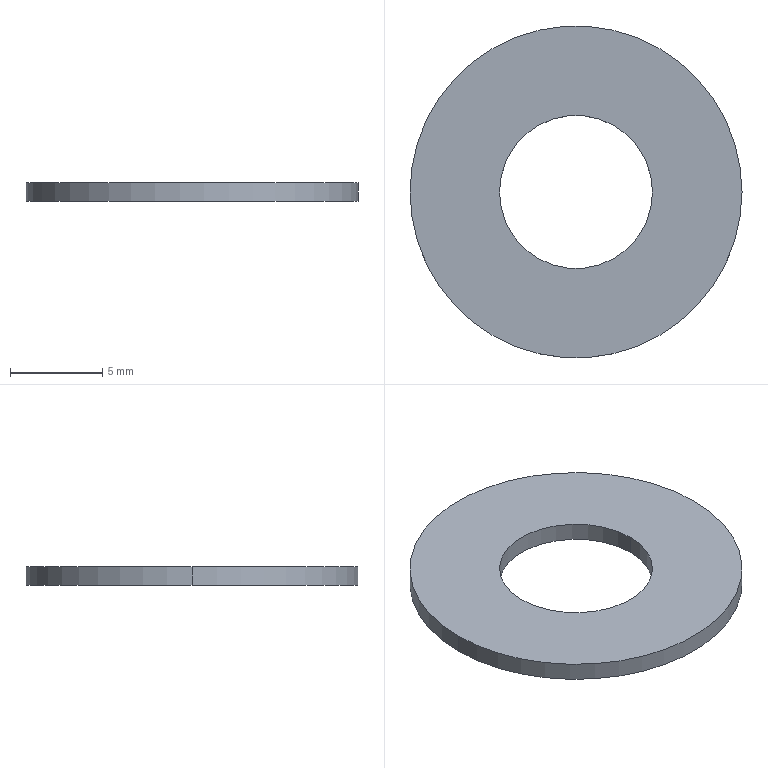Part | SolidWorks | features BaseBody 1 | 1 solid | 6 faces | box 18 x 18 x 1 mm | volume 200.363 mm3 | cylinder 4 | plane 2 | commonest cylinder face diameters 8.3 x2 18 x2
STEP:
#1=CARTESIAN_POINT('',(4.15,0.,1.));
#2=VERTEX_POINT('',#1);
#3=CARTESIAN_POINT('',(-4.15,0.,1.));
#4=VERTEX_POINT('',#3);
#5=CARTESIAN_POINT('',(0.,0.,1.));
#6=DIRECTION('',(0.,0.,-1.));
#7=DIRECTION('',(-1.,0.,0.));
#8=AXIS2_PLACEMENT_3D('',#5,#6,#7);
#9=CIRCLE('',#8,4.15);
#10=EDGE_CURVE('',#2,#4,#9,.T.);
#11=ORIENTED_EDGE('',*,*,#10,.F.);
#12=CARTESIAN_POINT('',(4.15,0.,0.));
#13=VERTEX_POINT('',#12);
#14=CARTESIAN_POINT('',(4.15,0.,1.));
#15=DIRECTION('',(0.,0.,-1.));
#16=VECTOR('',#15,1000.);
#17=LINE('',#14,#16);
#18=EDGE_CURVE('',#2,#13,#17,.T.);
#19=ORIENTED_EDGE('',*,*,#18,.T.);
#20=CARTESIAN_POINT('',(-4.15,0.,0.));
#21=VERTEX_POINT('',#20);
#22=CARTESIAN_POINT('',(0.,0.,0.));
#23=DIRECTION('',(0.,0.,1.));
#24=DIRECTION('',(-1.,0.,0.));
#25=AXIS2_PLACEMENT_3D('',#22,#23,#24);
#26=CIRCLE('',#25,4.15);
#27=EDGE_CURVE('',#21,#13,#26,.T.);
#28=ORIENTED_EDGE('',*,*,#27,.F.);
#29=CARTESIAN_POINT('',(-4.15,0.,1.));
#30=DIRECTION('',(0.,0.,-1.));
#31=VECTOR('',#30,1000.);
#32=LINE('',#29,#31);
#33=EDGE_CURVE('',#4,#21,#32,.T.);
#34=ORIENTED_EDGE('',*,*,#33,.F.);
#35=EDGE_LOOP('',(#11,#19,#28,#34));
#36=FACE_OUTER_BOUND('',#35,.T.);
#37=CARTESIAN_POINT('',(0.,0.,1.));
#38=DIRECTION('',(0.,0.,-1.));
#39=DIRECTION('',(-1.,0.,0.));
#40=AXIS2_PLACEMENT_3D('',#37,#38,#39);
#41=CYLINDRICAL_SURFACE('',#40,4.15);
#42=ADVANCED_FACE('',(#36),#41,.F.);
#43=CARTESIAN_POINT('',(9.,0.,1.));
#44=VERTEX_POINT('',#43);
#45=CARTESIAN_POINT('',(-9.,0.,1.));
#46=VERTEX_POINT('',#45);
#47=CARTESIAN_POINT('',(0.,0.,1.));
#48=DIRECTION('',(0.,0.,1.));
#49=DIRECTION('',(-1.,0.,0.));
#50=AXIS2_PLACEMENT_3D('',#47,#48,#49);
#51=CIRCLE('',#50,9.);
#52=EDGE_CURVE('',#44,#46,#51,.T.);
#53=ORIENTED_EDGE('',*,*,#52,.F.);
#54=CARTESIAN_POINT('',(9.,0.,0.));
#55=VERTEX_POINT('',#54);
#56=CARTESIAN_POINT('',(9.,0.,1.));
#57=DIRECTION('',(0.,0.,-1.));
#58=VECTOR('',#57,1000.);
#59=LINE('',#56,#58);
#60=EDGE_CURVE('',#44,#55,#59,.T.);
#61=ORIENTED_EDGE('',*,*,#60,.T.);
#62=CARTESIAN_POINT('',(-9.,0.,0.));
#63=VERTEX_POINT('',#62);
#64=CARTESIAN_POINT('',(0.,0.,0.));
#65=DIRECTION('',(0.,0.,1.));
#66=DIRECTION('',(-1.,0.,0.));
#67=AXIS2_PLACEMENT_3D('',#64,#65,#66);
#68=CIRCLE('',#67,9.);
#69=EDGE_CURVE('',#55,#63,#68,.T.);
#70=ORIENTED_EDGE('',*,*,#69,.T.);
#71=CARTESIAN_POINT('',(-9.,0.,1.));
#72=DIRECTION('',(0.,0.,-1.));
#73=VECTOR('',#72,1000.);
#74=LINE('',#71,#73);
#75=EDGE_CURVE('',#46,#63,#74,.T.);
#76=ORIENTED_EDGE('',*,*,#75,.F.);
#77=EDGE_LOOP('',(#53,#61,#70,#76));
#78=FACE_OUTER_BOUND('',#77,.T.);
#79=CARTESIAN_POINT('',(0.,0.,1.));
#80=DIRECTION('',(0.,0.,-1.));
#81=DIRECTION('',(-1.,0.,0.));
#82=AXIS2_PLACEMENT_3D('',#79,#80,#81);
#83=CYLINDRICAL_SURFACE('',#82,9.);
#84=ADVANCED_FACE('',(#78),#83,.T.);
#85=CARTESIAN_POINT('',(0.,0.,1.));
#86=DIRECTION('',(0.,0.,-1.));
#87=DIRECTION('',(-1.,0.,0.));
#88=AXIS2_PLACEMENT_3D('',#85,#86,#87);
#89=CIRCLE('',#88,4.15);
#90=EDGE_CURVE('',#4,#2,#89,.T.);
#91=ORIENTED_EDGE('',*,*,#90,.T.);
#92=ORIENTED_EDGE('',*,*,#10,.T.);
#93=EDGE_LOOP('',(#91,#92));
#94=FACE_BOUND('',#93,.T.);
#95=CARTESIAN_POINT('',(0.,0.,1.));
#96=DIRECTION('',(0.,0.,1.));
#97=DIRECTION('',(-1.,0.,0.));
#98=AXIS2_PLACEMENT_3D('',#95,#96,#97);
#99=CIRCLE('',#98,9.);
#100=EDGE_CURVE('',#46,#44,#99,.T.);
#101=ORIENTED_EDGE('',*,*,#100,.T.);
#102=ORIENTED_EDGE('',*,*,#52,.T.);
#103=EDGE_LOOP('',(#101,#102));
#104=FACE_OUTER_BOUND('',#103,.T.);
#105=CARTESIAN_POINT('',(0.,0.,1.));
#106=DIRECTION('',(0.,0.,1.));
#107=DIRECTION('',(1.,0.,0.));
#108=AXIS2_PLACEMENT_3D('',#105,#106,#107);
#109=PLANE('',#108);
#110=ADVANCED_FACE('',(#94,#104),#109,.T.);
#111=ORIENTED_EDGE('',*,*,#18,.F.);
#112=ORIENTED_EDGE('',*,*,#90,.F.);
#113=ORIENTED_EDGE('',*,*,#33,.T.);
#114=CARTESIAN_POINT('',(0.,0.,0.));
#115=DIRECTION('',(0.,0.,1.));
#116=DIRECTION('',(-1.,0.,0.));
#117=AXIS2_PLACEMENT_3D('',#114,#115,#116);
#118=CIRCLE('',#117,4.15);
#119=EDGE_CURVE('',#13,#21,#118,.T.);
#120=ORIENTED_EDGE('',*,*,#119,.F.);
#121=EDGE_LOOP('',(#111,#112,#113,#120));
#122=FACE_OUTER_BOUND('',#121,.T.);
#123=CARTESIAN_POINT('',(0.,0.,1.));
#124=DIRECTION('',(0.,0.,-1.));
#125=DIRECTION('',(-1.,0.,0.));
#126=AXIS2_PLACEMENT_3D('',#123,#124,#125);
#127=CYLINDRICAL_SURFACE('',#126,4.15);
#128=ADVANCED_FACE('',(#122),#127,.F.);
#129=ORIENTED_EDGE('',*,*,#60,.F.);
#130=ORIENTED_EDGE('',*,*,#100,.F.);
#131=ORIENTED_EDGE('',*,*,#75,.T.);
#132=CARTESIAN_POINT('',(0.,0.,0.));
#133=DIRECTION('',(0.,0.,1.));
#134=DIRECTION('',(-1.,0.,0.));
#135=AXIS2_PLACEMENT_3D('',#132,#133,#134);
#136=CIRCLE('',#135,9.);
#137=EDGE_CURVE('',#63,#55,#136,.T.);
#138=ORIENTED_EDGE('',*,*,#137,.T.);
#139=EDGE_LOOP('',(#129,#130,#131,#138));
#140=FACE_OUTER_BOUND('',#139,.T.);
#141=CARTESIAN_POINT('',(0.,0.,1.));
#142=DIRECTION('',(0.,0.,-1.));
#143=DIRECTION('',(-1.,0.,0.));
#144=AXIS2_PLACEMENT_3D('',#141,#142,#143);
#145=CYLINDRICAL_SURFACE('',#144,9.);
#146=ADVANCED_FACE('',(#140),#145,.T.);
#147=ORIENTED_EDGE('',*,*,#27,.T.);
#148=ORIENTED_EDGE('',*,*,#119,.T.);
#149=EDGE_LOOP('',(#147,#148));
#150=FACE_BOUND('',#149,.T.);
#151=ORIENTED_EDGE('',*,*,#137,.F.);
#152=ORIENTED_EDGE('',*,*,#69,.F.);
#153=EDGE_LOOP('',(#151,#152));
#154=FACE_OUTER_BOUND('',#153,.T.);
#155=CARTESIAN_POINT('',(0.,0.,0.));
#156=DIRECTION('',(0.,0.,1.));
#157=DIRECTION('',(1.,0.,0.));
#158=AXIS2_PLACEMENT_3D('',#155,#156,#157);
#159=PLANE('',#158);
#160=ADVANCED_FACE('',(#150,#154),#159,.F.);
#161=CLOSED_SHELL('',(#42,#84,#110,#128,#146,#160));
#162=MANIFOLD_SOLID_BREP('',#161);
#163=CARTESIAN_POINT('',(0.,0.,0.));
#164=DIRECTION('',(0.,0.,1.));
#165=DIRECTION('',(1.,0.,0.));
#166=AXIS2_PLACEMENT_3D('',#163,#164,#165);
#167=(LENGTH_UNIT()NAMED_UNIT(*)SI_UNIT(.MILLI.,.METRE.));
#168=UNCERTAINTY_MEASURE_WITH_UNIT(LENGTH_MEASURE(0.00001),#167,'','');
#169=(NAMED_UNIT(*)PLANE_ANGLE_UNIT()SI_UNIT($,.RADIAN.));
#170=(NAMED_UNIT(*)SI_UNIT($,.STERADIAN.)SOLID_ANGLE_UNIT());
#171=(GEOMETRIC_REPRESENTATION_CONTEXT(3)GLOBAL_UNCERTAINTY_ASSIGNED_CONTEXT((#168))GLOBAL_UNIT_ASSIGNED_CONTEXT((#167,#169,#170))REPRESENTATION_CONTEXT('',''));
#172=ADVANCED_BREP_SHAPE_REPRESENTATION('',(#162,#166),#171);